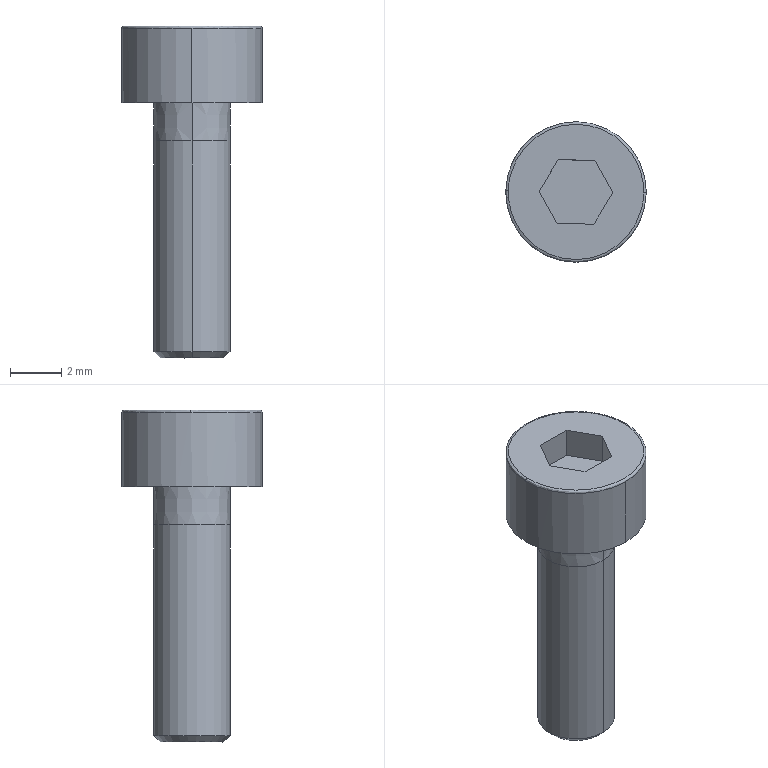Part | SolidWorks | features BaseBody 1 | 1 solid | 23 faces | box 5.5 x 5.5 x 13 mm | volume 134.337 mm3 | plane 11 | cylinder 6 | cone 4 | spline 2 | commonest cylinder face diameters 3 x2 3.2 x2 5.5 x2
STEP:
#1=CARTESIAN_POINT('',(510.512,-10.442,320.269));
#2=VERTEX_POINT('',#1);
#3=CARTESIAN_POINT('',(513.262,-7.733,320.269));
#4=VERTEX_POINT('',#3);
#5=CARTESIAN_POINT('',(513.262,-10.483,320.269));
#6=DIRECTION('',(0.000000003,0.000000008,-1.));
#7=DIRECTION('',(0.,1.,0.000000008));
#8=AXIS2_PLACEMENT_3D('',#5,#6,#7);
#9=CIRCLE('',#8,2.75);
#10=EDGE_CURVE('',#2,#4,#9,.T.);
#11=ORIENTED_EDGE('',*,*,#10,.F.);
#12=CARTESIAN_POINT('',(510.612,-10.443,320.369));
#13=VERTEX_POINT('',#12);
#14=CARTESIAN_POINT('',(510.612,-10.443,320.269));
#15=DIRECTION('',(0.01505,0.9999,0.000000008));
#16=DIRECTION('',(-0.9999,0.01505,-0.000000003));
#17=AXIS2_PLACEMENT_3D('',#14,#15,#16);
#18=CIRCLE('',#17,0.1);
#19=EDGE_CURVE('',#2,#13,#18,.T.);
#20=ORIENTED_EDGE('',*,*,#19,.T.);
#21=CARTESIAN_POINT('',(515.911,-10.523,320.369));
#22=VERTEX_POINT('',#21);
#23=CARTESIAN_POINT('',(510.612,-10.443,320.369));
#24=CARTESIAN_POINT('',(510.692,-5.144,320.369));
#25=CARTESIAN_POINT('',(515.991,-5.224,320.369));
#26=CARTESIAN_POINT('',(515.911,-10.523,320.369));
#27=(BOUNDED_CURVE()B_SPLINE_CURVE(3,(#23,#24,#25,#26),.UNSPECIFIED.,.F.,.F.)B_SPLINE_CURVE_WITH_KNOTS((4,4),(0.,1.),.UNSPECIFIED.)CURVE()GEOMETRIC_REPRESENTATION_ITEM()RATIONAL_B_SPLINE_CURVE((1.,0.3333,0.3333,1.))REPRESENTATION_ITEM(''));
#28=EDGE_CURVE('',#13,#22,#27,.T.);
#29=ORIENTED_EDGE('',*,*,#28,.T.);
#30=CARTESIAN_POINT('',(516.011,-10.525,320.269));
#31=VERTEX_POINT('',#30);
#32=CARTESIAN_POINT('',(515.911,-10.523,320.269));
#33=DIRECTION('',(-0.01505,-0.9999,-0.000000008));
#34=DIRECTION('',(0.9999,-0.01505,0.000000003));
#35=AXIS2_PLACEMENT_3D('',#32,#33,#34);
#36=CIRCLE('',#35,0.1);
#37=EDGE_CURVE('',#31,#22,#36,.T.);
#38=ORIENTED_EDGE('',*,*,#37,.F.);
#39=CARTESIAN_POINT('',(513.262,-10.483,320.269));
#40=DIRECTION('',(0.000000003,0.000000008,-1.));
#41=DIRECTION('',(0.,1.,0.000000008));
#42=AXIS2_PLACEMENT_3D('',#39,#40,#41);
#43=CIRCLE('',#42,2.75);
#44=EDGE_CURVE('',#4,#31,#43,.T.);
#45=ORIENTED_EDGE('',*,*,#44,.F.);
#46=EDGE_LOOP('',(#11,#20,#29,#38,#45));
#47=FACE_OUTER_BOUND('',#46,.T.);
#48=CARTESIAN_POINT('',(510.512,-10.442,320.269));
#49=CARTESIAN_POINT('',(510.595,-4.943,320.269));
#50=CARTESIAN_POINT('',(516.094,-5.025,320.269));
#51=CARTESIAN_POINT('',(516.011,-10.525,320.269));
#52=CARTESIAN_POINT('',(510.512,-10.442,320.328));
#53=CARTESIAN_POINT('',(510.595,-4.943,320.328));
#54=CARTESIAN_POINT('',(516.094,-5.025,320.328));
#55=CARTESIAN_POINT('',(516.011,-10.525,320.328));
#56=CARTESIAN_POINT('',(510.553,-10.443,320.369));
#57=CARTESIAN_POINT('',(510.635,-5.026,320.369));
#58=CARTESIAN_POINT('',(516.051,-5.108,320.369));
#59=CARTESIAN_POINT('',(515.97,-10.524,320.369));
#60=CARTESIAN_POINT('',(510.612,-10.443,320.369));
#61=CARTESIAN_POINT('',(510.692,-5.144,320.369));
#62=CARTESIAN_POINT('',(515.991,-5.224,320.369));
#63=CARTESIAN_POINT('',(515.911,-10.523,320.369));
#64=(BOUNDED_SURFACE()B_SPLINE_SURFACE(3,3,((#48,#49,#50,#51),(#52,#53,#54,#55),(#56,#57,#58,#59),(#60,#61,#62,#63)),.UNSPECIFIED.,.F.,.F.,.F.)B_SPLINE_SURFACE_WITH_KNOTS((4,4),(4,4),(0.,1.),(0.,1.),.UNSPECIFIED.)GEOMETRIC_REPRESENTATION_ITEM()RATIONAL_B_SPLINE_SURFACE(((1.,0.3333,0.3333,1.),(0.8047,0.2682,0.2682,0.8047),(0.8047,0.2682,0.2682,0.8047),(1.,0.3333,0.3333,1.)))REPRESENTATION_ITEM('')SURFACE());
#65=ADVANCED_FACE('',(#47),#64,.T.);
#66=CARTESIAN_POINT('',(513.262,-8.983,315.869));
#67=VERTEX_POINT('',#66);
#68=CARTESIAN_POINT('',(513.262,-11.983,315.869));
#69=VERTEX_POINT('',#68);
#70=CARTESIAN_POINT('',(513.262,-10.483,315.869));
#71=DIRECTION('',(0.000000003,0.000000008,-1.));
#72=DIRECTION('',(0.,1.,0.000000008));
#73=AXIS2_PLACEMENT_3D('',#70,#71,#72);
#74=CIRCLE('',#73,1.5);
#75=EDGE_CURVE('',#67,#69,#74,.T.);
#76=ORIENTED_EDGE('',*,*,#75,.T.);
#77=CARTESIAN_POINT('',(513.262,-11.983,307.619));
#78=VERTEX_POINT('',#77);
#79=CARTESIAN_POINT('',(513.262,-11.983,311.744));
#80=DIRECTION('',(0.000000003,0.000000008,-1.));
#81=VECTOR('',#80,1000.);
#82=LINE('',#79,#81);
#83=EDGE_CURVE('',#69,#78,#82,.T.);
#84=ORIENTED_EDGE('',*,*,#83,.T.);
#85=CARTESIAN_POINT('',(513.262,-8.983,307.619));
#86=VERTEX_POINT('',#85);
#87=CARTESIAN_POINT('',(513.262,-10.483,307.619));
#88=DIRECTION('',(-0.000000003,-0.000000008,1.));
#89=DIRECTION('',(0.,1.,0.000000008));
#90=AXIS2_PLACEMENT_3D('',#87,#88,#89);
#91=CIRCLE('',#90,1.5);
#92=EDGE_CURVE('',#78,#86,#91,.T.);
#93=ORIENTED_EDGE('',*,*,#92,.T.);
#94=CARTESIAN_POINT('',(513.262,-8.983,311.744));
#95=DIRECTION('',(0.000000003,0.000000008,-1.));
#96=VECTOR('',#95,1000.);
#97=LINE('',#94,#96);
#98=EDGE_CURVE('',#67,#86,#97,.T.);
#99=ORIENTED_EDGE('',*,*,#98,.F.);
#100=EDGE_LOOP('',(#76,#84,#93,#99));
#101=FACE_OUTER_BOUND('',#100,.T.);
#102=CARTESIAN_POINT('',(513.262,-10.483,311.744));
#103=DIRECTION('',(0.000000003,0.000000008,-1.));
#104=DIRECTION('',(0.,1.,0.000000008));
#105=AXIS2_PLACEMENT_3D('',#102,#103,#104);
#106=CYLINDRICAL_SURFACE('',#105,1.5);
#107=ADVANCED_FACE('',(#101),#106,.T.);
#108=CARTESIAN_POINT('',(513.262,-8.984,317.369));
#109=VERTEX_POINT('',#108);
#110=CARTESIAN_POINT('',(513.262,-11.983,317.369));
#111=VERTEX_POINT('',#110);
#112=CARTESIAN_POINT('',(513.262,-10.483,317.369));
#113=DIRECTION('',(0.000000003,0.000000008,-1.));
#114=DIRECTION('',(0.,1.,0.000000008));
#115=AXIS2_PLACEMENT_3D('',#112,#113,#114);
#116=CIRCLE('',#115,1.499);
#117=EDGE_CURVE('',#109,#111,#116,.T.);
#118=ORIENTED_EDGE('',*,*,#117,.T.);
#119=CARTESIAN_POINT('',(513.262,-11.983,315.869));
#120=DIRECTION('',(0.000000003,-0.0005,-1.));
#121=VECTOR('',#120,1000.);
#122=LINE('',#119,#121);
#123=EDGE_CURVE('',#111,#69,#122,.T.);
#124=ORIENTED_EDGE('',*,*,#123,.T.);
#125=ORIENTED_EDGE('',*,*,#75,.F.);
#126=CARTESIAN_POINT('',(513.262,-8.983,315.869));
#127=DIRECTION('',(0.000000003,0.0005,-1.));
#128=VECTOR('',#127,1000.);
#129=LINE('',#126,#128);
#130=EDGE_CURVE('',#109,#67,#129,.T.);
#131=ORIENTED_EDGE('',*,*,#130,.F.);
#132=EDGE_LOOP('',(#118,#124,#125,#131));
#133=FACE_OUTER_BOUND('',#132,.T.);
#134=CARTESIAN_POINT('',(513.262,-10.483,315.869));
#135=DIRECTION('',(0.000000003,0.000000008,-1.));
#136=DIRECTION('',(0.,1.,0.000000008));
#137=AXIS2_PLACEMENT_3D('',#134,#135,#136);
#138=CONICAL_SURFACE('',#137,1.5,0.0005);
#139=ADVANCED_FACE('',(#133),#138,.T.);
#140=CARTESIAN_POINT('',(513.262,-11.733,307.369));
#141=VERTEX_POINT('',#140);
#142=CARTESIAN_POINT('',(513.262,-9.233,307.369));
#143=VERTEX_POINT('',#142);
#144=CARTESIAN_POINT('',(513.262,-10.483,307.369));
#145=DIRECTION('',(-0.000000003,-0.000000008,1.));
#146=DIRECTION('',(0.,-1.,-0.000000008));
#147=AXIS2_PLACEMENT_3D('',#144,#145,#146);
#148=CIRCLE('',#147,1.25);
#149=EDGE_CURVE('',#141,#143,#148,.T.);
#150=ORIENTED_EDGE('',*,*,#149,.T.);
#151=CARTESIAN_POINT('',(513.262,-8.983,307.619));
#152=DIRECTION('',(-0.000000002,0.7071,0.7071));
#153=VECTOR('',#152,1000.);
#154=LINE('',#151,#153);
#155=EDGE_CURVE('',#143,#86,#154,.T.);
#156=ORIENTED_EDGE('',*,*,#155,.T.);
#157=ORIENTED_EDGE('',*,*,#92,.F.);
#158=CARTESIAN_POINT('',(513.262,-11.983,307.619));
#159=DIRECTION('',(-0.000000002,-0.7071,0.7071));
#160=VECTOR('',#159,1000.);
#161=LINE('',#158,#160);
#162=EDGE_CURVE('',#141,#78,#161,.T.);
#163=ORIENTED_EDGE('',*,*,#162,.F.);
#164=EDGE_LOOP('',(#150,#156,#157,#163));
#165=FACE_OUTER_BOUND('',#164,.T.);
#166=CARTESIAN_POINT('',(513.262,-10.483,307.619));
#167=DIRECTION('',(-0.000000003,-0.000000008,1.));
#168=DIRECTION('',(0.,-1.,-0.000000008));
#169=AXIS2_PLACEMENT_3D('',#166,#167,#168);
#170=CONICAL_SURFACE('',#169,1.5,0.7854);
#171=ADVANCED_FACE('',(#165),#170,.T.);
#172=ORIENTED_EDGE('',*,*,#44,.T.);
#173=CARTESIAN_POINT('',(513.262,-13.233,320.269));
#174=VERTEX_POINT('',#173);
#175=CARTESIAN_POINT('',(513.262,-10.483,320.269));
#176=DIRECTION('',(0.000000003,0.000000008,-1.));
#177=DIRECTION('',(0.,1.,0.000000008));
#178=AXIS2_PLACEMENT_3D('',#175,#176,#177);
#179=CIRCLE('',#178,2.75);
#180=EDGE_CURVE('',#31,#174,#179,.T.);
#181=ORIENTED_EDGE('',*,*,#180,.T.);
#182=CARTESIAN_POINT('',(513.262,-13.233,317.369));
#183=VERTEX_POINT('',#182);
#184=CARTESIAN_POINT('',(513.262,-13.233,318.819));
#185=DIRECTION('',(0.000000003,0.000000008,-1.));
#186=VECTOR('',#185,1000.);
#187=LINE('',#184,#186);
#188=EDGE_CURVE('',#174,#183,#187,.T.);
#189=ORIENTED_EDGE('',*,*,#188,.T.);
#190=CARTESIAN_POINT('',(513.262,-7.733,317.369));
#191=VERTEX_POINT('',#190);
#192=CARTESIAN_POINT('',(513.262,-10.483,317.369));
#193=DIRECTION('',(0.000000003,0.000000008,-1.));
#194=DIRECTION('',(0.,1.,0.000000008));
#195=AXIS2_PLACEMENT_3D('',#192,#193,#194);
#196=CIRCLE('',#195,2.75);
#197=EDGE_CURVE('',#191,#183,#196,.T.);
#198=ORIENTED_EDGE('',*,*,#197,.F.);
#199=CARTESIAN_POINT('',(513.262,-7.733,318.819));
#200=DIRECTION('',(0.000000003,0.000000008,-1.));
#201=VECTOR('',#200,1000.);
#202=LINE('',#199,#201);
#203=EDGE_CURVE('',#4,#191,#202,.T.);
#204=ORIENTED_EDGE('',*,*,#203,.F.);
#205=EDGE_LOOP('',(#172,#181,#189,#198,#204));
#206=FACE_OUTER_BOUND('',#205,.T.);
#207=CARTESIAN_POINT('',(513.262,-10.483,318.819));
#208=DIRECTION('',(0.000000003,0.000000008,-1.));
#209=DIRECTION('',(0.,1.,0.000000008));
#210=AXIS2_PLACEMENT_3D('',#207,#208,#209);
#211=CYLINDRICAL_SURFACE('',#210,2.75);
#212=ADVANCED_FACE('',(#206),#211,.T.);
#213=CARTESIAN_POINT('',(513.262,-8.883,319.069));
#214=VERTEX_POINT('',#213);
#215=CARTESIAN_POINT('',(513.262,-12.083,319.069));
#216=VERTEX_POINT('',#215);
#217=CARTESIAN_POINT('',(513.262,-10.483,319.069));
#218=DIRECTION('',(-0.000000003,-0.000000008,1.));
#219=DIRECTION('',(0.,-1.,-0.000000008));
#220=AXIS2_PLACEMENT_3D('',#217,#218,#219);
#221=CIRCLE('',#220,1.6);
#222=EDGE_CURVE('',#214,#216,#221,.T.);
#223=ORIENTED_EDGE('',*,*,#222,.F.);
#224=CARTESIAN_POINT('',(513.262,-8.883,319.169));
#225=VERTEX_POINT('',#224);
#226=CARTESIAN_POINT('',(513.262,-8.883,319.119));
#227=DIRECTION('',(-0.000000003,-0.000000008,1.));
#228=VECTOR('',#227,1000.);
#229=LINE('',#226,#228);
#230=EDGE_CURVE('',#214,#225,#229,.T.);
#231=ORIENTED_EDGE('',*,*,#230,.T.);
#232=CARTESIAN_POINT('',(513.262,-12.083,319.169));
#233=VERTEX_POINT('',#232);
#234=CARTESIAN_POINT('',(513.262,-10.483,319.169));
#235=DIRECTION('',(-0.000000003,-0.000000008,1.));
#236=DIRECTION('',(0.,-1.,-0.000000008));
#237=AXIS2_PLACEMENT_3D('',#234,#235,#236);
#238=CIRCLE('',#237,1.6);
#239=EDGE_CURVE('',#225,#233,#238,.T.);
#240=ORIENTED_EDGE('',*,*,#239,.T.);
#241=CARTESIAN_POINT('',(513.262,-12.083,319.119));
#242=DIRECTION('',(-0.000000003,-0.000000008,1.));
#243=VECTOR('',#242,1000.);
#244=LINE('',#241,#243);
#245=EDGE_CURVE('',#216,#233,#244,.T.);
#246=ORIENTED_EDGE('',*,*,#245,.F.);
#247=EDGE_LOOP('',(#223,#231,#240,#246));
#248=FACE_OUTER_BOUND('',#247,.T.);
#249=CARTESIAN_POINT('',(513.262,-10.483,319.119));
#250=DIRECTION('',(-0.000000003,-0.000000008,1.));
#251=DIRECTION('',(0.,-1.,-0.000000008));
#252=AXIS2_PLACEMENT_3D('',#249,#250,#251);
#253=CYLINDRICAL_SURFACE('',#252,1.6);
#254=ADVANCED_FACE('',(#248),#253,.F.);
#255=ORIENTED_EDGE('',*,*,#83,.F.);
#256=CARTESIAN_POINT('',(513.262,-10.483,315.869));
#257=DIRECTION('',(0.000000003,0.000000008,-1.));
#258=DIRECTION('',(0.,1.,0.000000008));
#259=AXIS2_PLACEMENT_3D('',#256,#257,#258);
#260=CIRCLE('',#259,1.5);
#261=EDGE_CURVE('',#69,#67,#260,.T.);
#262=ORIENTED_EDGE('',*,*,#261,.T.);
#263=ORIENTED_EDGE('',*,*,#98,.T.);
#264=CARTESIAN_POINT('',(513.262,-10.483,307.619));
#265=DIRECTION('',(-0.000000003,-0.000000008,1.));
#266=DIRECTION('',(0.,1.,0.000000008));
#267=AXIS2_PLACEMENT_3D('',#264,#265,#266);
#268=CIRCLE('',#267,1.5);
#269=EDGE_CURVE('',#86,#78,#268,.T.);
#270=ORIENTED_EDGE('',*,*,#269,.T.);
#271=EDGE_LOOP('',(#255,#262,#263,#270));
#272=FACE_OUTER_BOUND('',#271,.T.);
#273=CARTESIAN_POINT('',(513.262,-10.483,311.744));
#274=DIRECTION('',(0.000000003,0.000000008,-1.));
#275=DIRECTION('',(0.,1.,0.000000008));
#276=AXIS2_PLACEMENT_3D('',#273,#274,#275);
#277=CYLINDRICAL_SURFACE('',#276,1.5);
#278=ADVANCED_FACE('',(#272),#277,.T.);
#279=ORIENTED_EDGE('',*,*,#123,.F.);
#280=CARTESIAN_POINT('',(513.262,-10.483,317.369));
#281=DIRECTION('',(0.000000003,0.000000008,-1.));
#282=DIRECTION('',(0.,1.,0.000000008));
#283=AXIS2_PLACEMENT_3D('',#280,#281,#282);
#284=CIRCLE('',#283,1.499);
#285=EDGE_CURVE('',#111,#109,#284,.T.);
#286=ORIENTED_EDGE('',*,*,#285,.T.);
#287=ORIENTED_EDGE('',*,*,#130,.T.);
#288=ORIENTED_EDGE('',*,*,#261,.F.);
#289=EDGE_LOOP('',(#279,#286,#287,#288));
#290=FACE_OUTER_BOUND('',#289,.T.);
#291=CARTESIAN_POINT('',(513.262,-10.483,315.869));
#292=DIRECTION('',(0.000000003,0.000000008,-1.));
#293=DIRECTION('',(0.,1.,0.000000008));
#294=AXIS2_PLACEMENT_3D('',#291,#292,#293);
#295=CONICAL_SURFACE('',#294,1.5,0.0005);
#296=ADVANCED_FACE('',(#290),#295,.T.);
#297=ORIENTED_EDGE('',*,*,#155,.F.);
#298=CARTESIAN_POINT('',(513.262,-10.483,307.369));
#299=DIRECTION('',(-0.000000003,-0.000000008,1.));
#300=DIRECTION('',(0.,-1.,-0.000000008));
#301=AXIS2_PLACEMENT_3D('',#298,#299,#300);
#302=CIRCLE('',#301,1.25);
#303=EDGE_CURVE('',#143,#141,#302,.T.);
#304=ORIENTED_EDGE('',*,*,#303,.T.);
#305=ORIENTED_EDGE('',*,*,#162,.T.);
#306=ORIENTED_EDGE('',*,*,#269,.F.);
#307=EDGE_LOOP('',(#297,#304,#305,#306));
#308=FACE_OUTER_BOUND('',#307,.T.);
#309=CARTESIAN_POINT('',(513.262,-10.483,307.619));
#310=DIRECTION('',(-0.000000003,-0.000000008,1.));
#311=DIRECTION('',(0.,-1.,-0.000000008));
#312=AXIS2_PLACEMENT_3D('',#309,#310,#311);
#313=CONICAL_SURFACE('',#312,1.5,0.7854);
#314=ADVANCED_FACE('',(#308),#313,.T.);
#315=ORIENTED_EDGE('',*,*,#117,.F.);
#316=ORIENTED_EDGE('',*,*,#285,.F.);
#317=EDGE_LOOP('',(#315,#316));
#318=FACE_BOUND('',#317,.T.);
#319=ORIENTED_EDGE('',*,*,#197,.T.);
#320=CARTESIAN_POINT('',(513.262,-10.483,317.369));
#321=DIRECTION('',(0.000000003,0.000000008,-1.));
#322=DIRECTION('',(0.,1.,0.000000008));
#323=AXIS2_PLACEMENT_3D('',#320,#321,#322);
#324=CIRCLE('',#323,2.75);
#325=EDGE_CURVE('',#183,#191,#324,.T.);
#326=ORIENTED_EDGE('',*,*,#325,.T.);
#327=EDGE_LOOP('',(#319,#326));
#328=FACE_OUTER_BOUND('',#327,.T.);
#329=CARTESIAN_POINT('',(514.636,-10.504,317.369));
#330=DIRECTION('',(0.000000003,0.000000008,-1.));
#331=DIRECTION('',(0.,1.,0.000000008));
#332=AXIS2_PLACEMENT_3D('',#329,#330,#331);
#333=PLANE('',#332);
#334=ADVANCED_FACE('',(#318,#328),#333,.T.);
#335=ORIENTED_EDGE('',*,*,#149,.F.);
#336=ORIENTED_EDGE('',*,*,#303,.F.);
#337=EDGE_LOOP('',(#335,#336));
#338=FACE_OUTER_BOUND('',#337,.T.);
#339=CARTESIAN_POINT('',(513.886,-10.493,307.369));
#340=DIRECTION('',(0.000000003,0.000000008,-1.));
#341=DIRECTION('',(0.,1.,0.000000008));
#342=AXIS2_PLACEMENT_3D('',#339,#340,#341);
#343=PLANE('',#342);
#344=ADVANCED_FACE('',(#338),#343,.T.);
#345=ORIENTED_EDGE('',*,*,#188,.F.);
#346=CARTESIAN_POINT('',(513.262,-10.483,320.269));
#347=DIRECTION('',(0.000000003,0.000000008,-1.));
#348=DIRECTION('',(0.,1.,0.000000008));
#349=AXIS2_PLACEMENT_3D('',#346,#347,#348);
#350=CIRCLE('',#349,2.75);
#351=EDGE_CURVE('',#174,#2,#350,.T.);
#352=ORIENTED_EDGE('',*,*,#351,.T.);
#353=ORIENTED_EDGE('',*,*,#10,.T.);
#354=ORIENTED_EDGE('',*,*,#203,.T.);
#355=ORIENTED_EDGE('',*,*,#325,.F.);
#356=EDGE_LOOP('',(#345,#352,#353,#354,#355));
#357=FACE_OUTER_BOUND('',#356,.T.);
#358=CARTESIAN_POINT('',(513.262,-10.483,318.819));
#359=DIRECTION('',(0.000000003,0.000000008,-1.));
#360=DIRECTION('',(0.,1.,0.000000008));
#361=AXIS2_PLACEMENT_3D('',#358,#359,#360);
#362=CYLINDRICAL_SURFACE('',#361,2.75);
#363=ADVANCED_FACE('',(#357),#362,.T.);
#364=ORIENTED_EDGE('',*,*,#19,.F.);
#365=ORIENTED_EDGE('',*,*,#351,.F.);
#366=ORIENTED_EDGE('',*,*,#180,.F.);
#367=ORIENTED_EDGE('',*,*,#37,.T.);
#368=CARTESIAN_POINT('',(515.911,-10.523,320.369));
#369=CARTESIAN_POINT('',(515.831,-15.823,320.369));
#370=CARTESIAN_POINT('',(510.532,-15.743,320.369));
#371=CARTESIAN_POINT('',(510.612,-10.443,320.369));
#372=(BOUNDED_CURVE()B_SPLINE_CURVE(3,(#368,#369,#370,#371),.UNSPECIFIED.,.F.,.F.)B_SPLINE_CURVE_WITH_KNOTS((4,4),(0.,1.),.UNSPECIFIED.)CURVE()GEOMETRIC_REPRESENTATION_ITEM()RATIONAL_B_SPLINE_CURVE((1.,0.3333,0.3333,1.))REPRESENTATION_ITEM(''));
#373=EDGE_CURVE('',#22,#13,#372,.T.);
#374=ORIENTED_EDGE('',*,*,#373,.T.);
#375=EDGE_LOOP('',(#364,#365,#366,#367,#374));
#376=FACE_OUTER_BOUND('',#375,.T.);
#377=CARTESIAN_POINT('',(516.011,-10.525,320.269));
#378=CARTESIAN_POINT('',(515.928,-16.024,320.269));
#379=CARTESIAN_POINT('',(510.429,-15.941,320.269));
#380=CARTESIAN_POINT('',(510.512,-10.442,320.269));
#381=CARTESIAN_POINT('',(516.011,-10.525,320.328));
#382=CARTESIAN_POINT('',(515.928,-16.024,320.328));
#383=CARTESIAN_POINT('',(510.429,-15.941,320.328));
#384=CARTESIAN_POINT('',(510.512,-10.442,320.328));
#385=CARTESIAN_POINT('',(515.97,-10.524,320.369));
#386=CARTESIAN_POINT('',(515.888,-15.941,320.369));
#387=CARTESIAN_POINT('',(510.472,-15.859,320.369));
#388=CARTESIAN_POINT('',(510.553,-10.443,320.369));
#389=CARTESIAN_POINT('',(515.911,-10.523,320.369));
#390=CARTESIAN_POINT('',(515.831,-15.823,320.369));
#391=CARTESIAN_POINT('',(510.532,-15.743,320.369));
#392=CARTESIAN_POINT('',(510.612,-10.443,320.369));
#393=(BOUNDED_SURFACE()B_SPLINE_SURFACE(3,3,((#377,#378,#379,#380),(#381,#382,#383,#384),(#385,#386,#387,#388),(#389,#390,#391,#392)),.UNSPECIFIED.,.F.,.F.,.F.)B_SPLINE_SURFACE_WITH_KNOTS((4,4),(4,4),(0.,1.),(0.,1.),.UNSPECIFIED.)GEOMETRIC_REPRESENTATION_ITEM()RATIONAL_B_SPLINE_SURFACE(((1.,0.3333,0.3333,1.),(0.8047,0.2682,0.2682,0.8047),(0.8047,0.2682,0.2682,0.8047),(1.,0.3333,0.3333,1.)))REPRESENTATION_ITEM('')SURFACE());
#394=ADVANCED_FACE('',(#376),#393,.T.);
#395=ORIENTED_EDGE('',*,*,#28,.F.);
#396=ORIENTED_EDGE('',*,*,#373,.F.);
#397=EDGE_LOOP('',(#395,#396));
#398=FACE_OUTER_BOUND('',#397,.T.);
#399=CARTESIAN_POINT('',(512.521,-11.722,320.369));
#400=VERTEX_POINT('',#399);
#401=CARTESIAN_POINT('',(511.818,-10.462,320.369));
#402=VERTEX_POINT('',#401);
#403=CARTESIAN_POINT('',(512.521,-11.722,320.369));
#404=DIRECTION('',(-0.4869,0.8735,0.000000006));
#405=VECTOR('',#404,1000.);
#406=LINE('',#403,#405);
#407=EDGE_CURVE('',#400,#402,#406,.T.);
#408=ORIENTED_EDGE('',*,*,#407,.T.);
#409=CARTESIAN_POINT('',(512.559,-9.223,320.369));
#410=VERTEX_POINT('',#409);
#411=CARTESIAN_POINT('',(511.818,-10.462,320.369));
#412=DIRECTION('',(0.513,0.8584,0.000000009));
#413=VECTOR('',#412,1000.);
#414=LINE('',#411,#413);
#415=EDGE_CURVE('',#402,#410,#414,.T.);
#416=ORIENTED_EDGE('',*,*,#415,.T.);
#417=CARTESIAN_POINT('',(514.002,-9.244,320.369));
#418=VERTEX_POINT('',#417);
#419=CARTESIAN_POINT('',(512.559,-9.223,320.369));
#420=DIRECTION('',(0.9999,-0.01505,0.000000003));
#421=VECTOR('',#420,1000.);
#422=LINE('',#419,#421);
#423=EDGE_CURVE('',#410,#418,#422,.T.);
#424=ORIENTED_EDGE('',*,*,#423,.T.);
#425=CARTESIAN_POINT('',(514.705,-10.505,320.369));
#426=VERTEX_POINT('',#425);
#427=CARTESIAN_POINT('',(514.002,-9.244,320.369));
#428=DIRECTION('',(0.4869,-0.8735,-0.000000006));
#429=VECTOR('',#428,1000.);
#430=LINE('',#427,#429);
#431=EDGE_CURVE('',#418,#426,#430,.T.);
#432=ORIENTED_EDGE('',*,*,#431,.T.);
#433=CARTESIAN_POINT('',(513.964,-11.744,320.369));
#434=VERTEX_POINT('',#433);
#435=CARTESIAN_POINT('',(514.705,-10.505,320.369));
#436=DIRECTION('',(-0.513,-0.8584,-0.000000009));
#437=VECTOR('',#436,1000.);
#438=LINE('',#435,#437);
#439=EDGE_CURVE('',#426,#434,#438,.T.);
#440=ORIENTED_EDGE('',*,*,#439,.T.);
#441=CARTESIAN_POINT('',(513.964,-11.744,320.369));
#442=DIRECTION('',(-0.9999,0.01505,-0.000000003));
#443=VECTOR('',#442,1000.);
#444=LINE('',#441,#443);
#445=EDGE_CURVE('',#434,#400,#444,.T.);
#446=ORIENTED_EDGE('',*,*,#445,.T.);
#447=EDGE_LOOP('',(#408,#416,#424,#432,#440,#446));
#448=FACE_BOUND('',#447,.T.);
#449=CARTESIAN_POINT('',(514.586,-10.503,320.369));
#450=DIRECTION('',(-0.000000003,-0.000000008,1.));
#451=DIRECTION('',(0.,-1.,-0.000000008));
#452=AXIS2_PLACEMENT_3D('',#449,#450,#451);
#453=PLANE('',#452);
#454=ADVANCED_FACE('',(#398,#448),#453,.T.);
#455=CARTESIAN_POINT('',(512.559,-9.223,319.169));
#456=VERTEX_POINT('',#455);
#457=CARTESIAN_POINT('',(512.559,-9.223,320.369));
#458=DIRECTION('',(-0.000000002,0.000000001,-1.));
#459=VECTOR('',#458,1000.);
#460=LINE('',#457,#459);
#461=EDGE_CURVE('',#410,#456,#460,.T.);
#462=ORIENTED_EDGE('',*,*,#461,.F.);
#463=ORIENTED_EDGE('',*,*,#415,.F.);
#464=CARTESIAN_POINT('',(511.818,-10.462,319.169));
#465=VERTEX_POINT('',#464);
#466=CARTESIAN_POINT('',(511.818,-10.462,320.369));
#467=DIRECTION('',(0.000000002,-0.000000001,1.));
#468=VECTOR('',#467,1000.);
#469=LINE('',#466,#468);
#470=EDGE_CURVE('',#465,#402,#469,.T.);
#471=ORIENTED_EDGE('',*,*,#470,.F.);
#472=CARTESIAN_POINT('',(512.559,-9.223,319.169));
#473=DIRECTION('',(-0.513,-0.8584,0.));
#474=VECTOR('',#473,1000.);
#475=LINE('',#472,#474);
#476=EDGE_CURVE('',#456,#465,#475,.T.);
#477=ORIENTED_EDGE('',*,*,#476,.F.);
#478=EDGE_LOOP('',(#462,#463,#471,#477));
#479=FACE_OUTER_BOUND('',#478,.T.);
#480=CARTESIAN_POINT('',(512.559,-9.223,320.369));
#481=DIRECTION('',(-0.8584,0.513,0.000000002));
#482=DIRECTION('',(-0.513,-0.8584,0.));
#483=AXIS2_PLACEMENT_3D('',#480,#481,#482);
#484=PLANE('',#483);
#485=ADVANCED_FACE('',(#479),#484,.F.);
#486=ORIENTED_EDGE('',*,*,#470,.T.);
#487=ORIENTED_EDGE('',*,*,#407,.F.);
#488=CARTESIAN_POINT('',(512.521,-11.722,319.169));
#489=VERTEX_POINT('',#488);
#490=CARTESIAN_POINT('',(512.521,-11.722,320.369));
#491=DIRECTION('',(-0.000000006,-0.000000003,1.));
#492=VECTOR('',#491,1000.);
#493=LINE('',#490,#492);
#494=EDGE_CURVE('',#489,#400,#493,.T.);
#495=ORIENTED_EDGE('',*,*,#494,.F.);
#496=CARTESIAN_POINT('',(511.818,-10.462,319.169));
#497=DIRECTION('',(0.4869,-0.8735,0.));
#498=VECTOR('',#497,1000.);
#499=LINE('',#496,#498);
#500=EDGE_CURVE('',#465,#489,#499,.T.);
#501=ORIENTED_EDGE('',*,*,#500,.F.);
#502=EDGE_LOOP('',(#486,#487,#495,#501));
#503=FACE_OUTER_BOUND('',#502,.T.);
#504=CARTESIAN_POINT('',(511.818,-10.462,320.369));
#505=DIRECTION('',(-0.8735,-0.4869,-0.000000007));
#506=DIRECTION('',(0.4869,-0.8735,0.));
#507=AXIS2_PLACEMENT_3D('',#504,#505,#506);
#508=PLANE('',#507);
#509=ADVANCED_FACE('',(#503),#508,.F.);
#510=ORIENTED_EDGE('',*,*,#494,.T.);
#511=ORIENTED_EDGE('',*,*,#445,.F.);
#512=CARTESIAN_POINT('',(513.964,-11.744,319.169));
#513=VERTEX_POINT('',#512);
#514=CARTESIAN_POINT('',(513.964,-11.744,320.369));
#515=DIRECTION('',(0.,-0.000000008,1.));
#516=VECTOR('',#515,1000.);
#517=LINE('',#514,#516);
#518=EDGE_CURVE('',#513,#434,#517,.T.);
#519=ORIENTED_EDGE('',*,*,#518,.F.);
#520=CARTESIAN_POINT('',(512.521,-11.722,319.169));
#521=DIRECTION('',(0.9999,-0.01505,0.));
#522=VECTOR('',#521,1000.);
#523=LINE('',#520,#522);
#524=EDGE_CURVE('',#489,#513,#523,.T.);
#525=ORIENTED_EDGE('',*,*,#524,.F.);
#526=EDGE_LOOP('',(#510,#511,#519,#525));
#527=FACE_OUTER_BOUND('',#526,.T.);
#528=CARTESIAN_POINT('',(512.521,-11.722,320.369));
#529=DIRECTION('',(-0.01505,-0.9999,-0.000000008));
#530=DIRECTION('',(0.9999,-0.01505,0.));
#531=AXIS2_PLACEMENT_3D('',#528,#529,#530);
#532=PLANE('',#531);
#533=ADVANCED_FACE('',(#527),#532,.F.);
#534=ORIENTED_EDGE('',*,*,#518,.T.);
#535=ORIENTED_EDGE('',*,*,#439,.F.);
#536=CARTESIAN_POINT('',(514.705,-10.505,319.169));
#537=VERTEX_POINT('',#536);
#538=CARTESIAN_POINT('',(514.705,-10.505,320.369));
#539=DIRECTION('',(0.000000002,-0.000000001,1.));
#540=VECTOR('',#539,1000.);
#541=LINE('',#538,#540);
#542=EDGE_CURVE('',#537,#426,#541,.T.);
#543=ORIENTED_EDGE('',*,*,#542,.F.);
#544=CARTESIAN_POINT('',(513.964,-11.744,319.169));
#545=DIRECTION('',(0.513,0.8584,0.));
#546=VECTOR('',#545,1000.);
#547=LINE('',#544,#546);
#548=EDGE_CURVE('',#513,#537,#547,.T.);
#549=ORIENTED_EDGE('',*,*,#548,.F.);
#550=EDGE_LOOP('',(#534,#535,#543,#549));
#551=FACE_OUTER_BOUND('',#550,.T.);
#552=CARTESIAN_POINT('',(513.964,-11.744,320.369));
#553=DIRECTION('',(0.8584,-0.513,-0.000000002));
#554=DIRECTION('',(0.513,0.8584,0.));
#555=AXIS2_PLACEMENT_3D('',#552,#553,#554);
#556=PLANE('',#555);
#557=ADVANCED_FACE('',(#551),#556,.F.);
#558=ORIENTED_EDGE('',*,*,#542,.T.);
#559=ORIENTED_EDGE('',*,*,#431,.F.);
#560=CARTESIAN_POINT('',(514.002,-9.244,319.169));
#561=VERTEX_POINT('',#560);
#562=CARTESIAN_POINT('',(514.002,-9.244,320.369));
#563=DIRECTION('',(-0.000000006,-0.000000003,1.));
#564=VECTOR('',#563,1000.);
#565=LINE('',#562,#564);
#566=EDGE_CURVE('',#561,#418,#565,.T.);
#567=ORIENTED_EDGE('',*,*,#566,.F.);
#568=CARTESIAN_POINT('',(514.705,-10.505,319.169));
#569=DIRECTION('',(-0.4869,0.8735,0.));
#570=VECTOR('',#569,1000.);
#571=LINE('',#568,#570);
#572=EDGE_CURVE('',#537,#561,#571,.T.);
#573=ORIENTED_EDGE('',*,*,#572,.F.);
#574=EDGE_LOOP('',(#558,#559,#567,#573));
#575=FACE_OUTER_BOUND('',#574,.T.);
#576=CARTESIAN_POINT('',(514.705,-10.505,320.369));
#577=DIRECTION('',(0.8735,0.4869,0.000000007));
#578=DIRECTION('',(-0.4869,0.8735,0.));
#579=AXIS2_PLACEMENT_3D('',#576,#577,#578);
#580=PLANE('',#579);
#581=ADVANCED_FACE('',(#575),#580,.F.);
#582=ORIENTED_EDGE('',*,*,#566,.T.);
#583=ORIENTED_EDGE('',*,*,#423,.F.);
#584=ORIENTED_EDGE('',*,*,#461,.T.);
#585=CARTESIAN_POINT('',(514.002,-9.244,319.169));
#586=DIRECTION('',(-0.9999,0.01505,0.));
#587=VECTOR('',#586,1000.);
#588=LINE('',#585,#587);
#589=EDGE_CURVE('',#561,#456,#588,.T.);
#590=ORIENTED_EDGE('',*,*,#589,.F.);
#591=EDGE_LOOP('',(#582,#583,#584,#590));
#592=FACE_OUTER_BOUND('',#591,.T.);
#593=CARTESIAN_POINT('',(514.002,-9.244,320.369));
#594=DIRECTION('',(0.01505,0.9999,0.000000008));
#595=DIRECTION('',(-0.9999,0.01505,0.));
#596=AXIS2_PLACEMENT_3D('',#593,#594,#595);
#597=PLANE('',#596);
#598=ADVANCED_FACE('',(#592),#597,.F.);
#599=CARTESIAN_POINT('',(513.262,-10.483,319.169));
#600=DIRECTION('',(-0.000000003,-0.000000008,1.));
#601=DIRECTION('',(0.,-1.,-0.000000008));
#602=AXIS2_PLACEMENT_3D('',#599,#600,#601);
#603=CIRCLE('',#602,1.6);
#604=EDGE_CURVE('',#233,#225,#603,.T.);
#605=ORIENTED_EDGE('',*,*,#604,.F.);
#606=ORIENTED_EDGE('',*,*,#239,.F.);
#607=EDGE_LOOP('',(#605,#606));
#608=FACE_OUTER_BOUND('',#607,.T.);
#609=ORIENTED_EDGE('',*,*,#476,.T.);
#610=ORIENTED_EDGE('',*,*,#500,.T.);
#611=ORIENTED_EDGE('',*,*,#524,.T.);
#612=ORIENTED_EDGE('',*,*,#548,.T.);
#613=ORIENTED_EDGE('',*,*,#572,.T.);
#614=ORIENTED_EDGE('',*,*,#589,.T.);
#615=EDGE_LOOP('',(#609,#610,#611,#612,#613,#614));
#616=FACE_BOUND('',#615,.T.);
#617=CARTESIAN_POINT('',(514.061,-10.495,319.169));
#618=DIRECTION('',(-0.000000003,-0.000000008,1.));
#619=DIRECTION('',(0.,-1.,-0.000000008));
#620=AXIS2_PLACEMENT_3D('',#617,#618,#619);
#621=PLANE('',#620);
#622=ADVANCED_FACE('',(#608,#616),#621,.F.);
#623=ORIENTED_EDGE('',*,*,#230,.F.);
#624=CARTESIAN_POINT('',(513.262,-10.483,319.069));
#625=DIRECTION('',(-0.000000003,-0.000000008,1.));
#626=DIRECTION('',(0.,-1.,-0.000000008));
#627=AXIS2_PLACEMENT_3D('',#624,#625,#626);
#628=CIRCLE('',#627,1.6);
#629=EDGE_CURVE('',#216,#214,#628,.T.);
#630=ORIENTED_EDGE('',*,*,#629,.F.);
#631=ORIENTED_EDGE('',*,*,#245,.T.);
#632=ORIENTED_EDGE('',*,*,#604,.T.);
#633=EDGE_LOOP('',(#623,#630,#631,#632));
#634=FACE_OUTER_BOUND('',#633,.T.);
#635=CARTESIAN_POINT('',(513.262,-10.483,319.119));
#636=DIRECTION('',(-0.000000003,-0.000000008,1.));
#637=DIRECTION('',(0.,-1.,-0.000000008));
#638=AXIS2_PLACEMENT_3D('',#635,#636,#637);
#639=CYLINDRICAL_SURFACE('',#638,1.6);
#640=ADVANCED_FACE('',(#634),#639,.F.);
#641=ORIENTED_EDGE('',*,*,#629,.T.);
#642=ORIENTED_EDGE('',*,*,#222,.T.);
#643=EDGE_LOOP('',(#641,#642));
#644=FACE_OUTER_BOUND('',#643,.T.);
#645=CARTESIAN_POINT('',(513.262,-10.483,319.069));
#646=DIRECTION('',(-0.000000003,-0.000000008,1.));
#647=DIRECTION('',(0.,-1.,-0.000000008));
#648=AXIS2_PLACEMENT_3D('',#645,#646,#647);
#649=PLANE('',#648);
#650=ADVANCED_FACE('',(#644),#649,.T.);
#651=CLOSED_SHELL('',(#65,#107,#139,#171,#212,#254,#278,#296,#314,#334,#344,#363,#394,#454,#485,#509,#533,#557,#581,#598,#622,#640,#650));
#652=MANIFOLD_SOLID_BREP('',#651);
#653=CARTESIAN_POINT('',(0.,0.,0.));
#654=DIRECTION('',(0.,0.,1.));
#655=DIRECTION('',(1.,0.,0.));
#656=AXIS2_PLACEMENT_3D('',#653,#654,#655);
#657=(LENGTH_UNIT()NAMED_UNIT(*)SI_UNIT(.MILLI.,.METRE.));
#658=UNCERTAINTY_MEASURE_WITH_UNIT(LENGTH_MEASURE(0.00001),#657,'','');
#659=(NAMED_UNIT(*)PLANE_ANGLE_UNIT()SI_UNIT($,.RADIAN.));
#660=(NAMED_UNIT(*)SI_UNIT($,.STERADIAN.)SOLID_ANGLE_UNIT());
#661=(GEOMETRIC_REPRESENTATION_CONTEXT(3)GLOBAL_UNCERTAINTY_ASSIGNED_CONTEXT((#658))GLOBAL_UNIT_ASSIGNED_CONTEXT((#657,#659,#660))REPRESENTATION_CONTEXT('',''));
#662=ADVANCED_BREP_SHAPE_REPRESENTATION('',(#652,#656),#661);